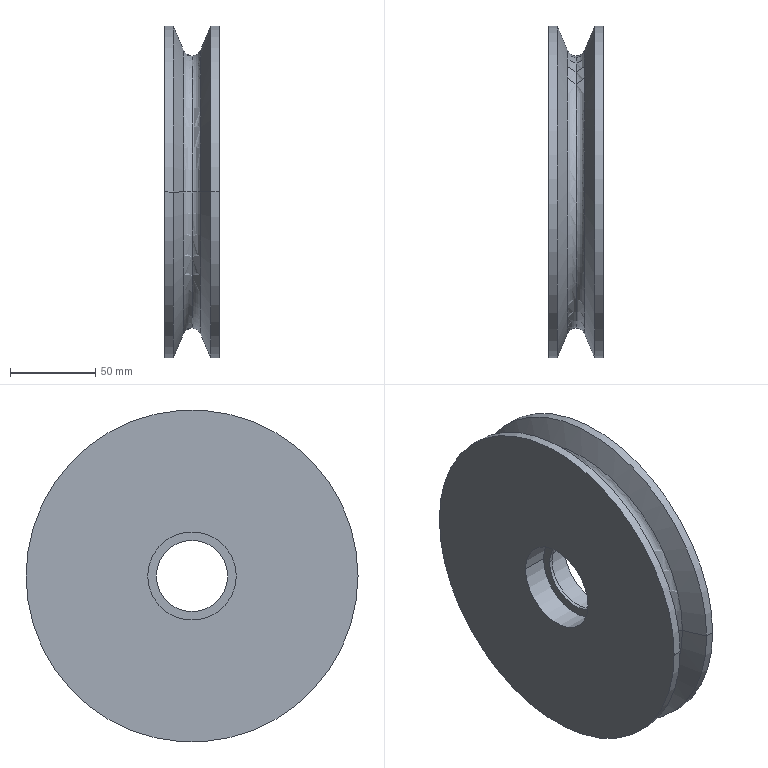Part | SolidWorks | features ICE 2, MirrorPattern 1, Revolution 1 | 1 solid | 22 faces | box 32 x 195 x 195 mm | volume 746203 mm3 | cylinder 10 | torus 4 | cone 4 | plane 4 | commonest cylinder face diameters 52 x4 195 x4 42 x2
STEP:
#1=CARTESIAN_POINT('',(5.072,83.372,0.));
#2=VERTEX_POINT('',#1);
#3=CARTESIAN_POINT('',(0.,80.,0.));
#4=VERTEX_POINT('',#3);
#5=CARTESIAN_POINT('',(0.,85.5,0.));
#6=DIRECTION('',(0.,0.,-1.));
#7=DIRECTION('',(-1.,0.,0.));
#8=AXIS2_PLACEMENT_3D('',#5,#6,#7);
#9=CIRCLE('',#8,5.5);
#10=EDGE_CURVE('',#2,#4,#9,.T.);
#11=ORIENTED_EDGE('',*,*,#10,.T.);
#12=CARTESIAN_POINT('',(0.,-80.,0.));
#13=VERTEX_POINT('',#12);
#14=CARTESIAN_POINT('',(0.,0.,0.));
#15=DIRECTION('',(1.,0.,0.));
#16=DIRECTION('',(0.,1.,0.));
#17=AXIS2_PLACEMENT_3D('',#14,#15,#16);
#18=CIRCLE('',#17,80.);
#19=EDGE_CURVE('',#4,#13,#18,.T.);
#20=ORIENTED_EDGE('',*,*,#19,.T.);
#21=CARTESIAN_POINT('',(5.072,-83.372,0.));
#22=VERTEX_POINT('',#21);
#23=CARTESIAN_POINT('',(0.,-85.5,0.));
#24=DIRECTION('',(0.,0.,1.));
#25=DIRECTION('',(0.,-1.,0.));
#26=AXIS2_PLACEMENT_3D('',#23,#24,#25);
#27=CIRCLE('',#26,5.5);
#28=EDGE_CURVE('',#22,#13,#27,.T.);
#29=ORIENTED_EDGE('',*,*,#28,.F.);
#30=CARTESIAN_POINT('',(5.072,0.,0.));
#31=DIRECTION('',(1.,0.,0.));
#32=DIRECTION('',(0.,1.,0.));
#33=AXIS2_PLACEMENT_3D('',#30,#31,#32);
#34=CIRCLE('',#33,83.372);
#35=EDGE_CURVE('',#2,#22,#34,.T.);
#36=ORIENTED_EDGE('',*,*,#35,.F.);
#37=EDGE_LOOP('',(#11,#20,#29,#36));
#38=FACE_OUTER_BOUND('',#37,.T.);
#39=CARTESIAN_POINT('',(0.,0.,0.));
#40=DIRECTION('',(1.,0.,0.));
#41=DIRECTION('',(0.,1.,0.));
#42=AXIS2_PLACEMENT_3D('',#39,#40,#41);
#43=TOROIDAL_SURFACE('',#42,85.5,5.5);
#44=ADVANCED_FACE('',(#38),#43,.F.);
#45=ORIENTED_EDGE('',*,*,#28,.T.);
#46=CARTESIAN_POINT('',(0.,0.,0.));
#47=DIRECTION('',(1.,0.,0.));
#48=DIRECTION('',(0.,1.,0.));
#49=AXIS2_PLACEMENT_3D('',#46,#47,#48);
#50=CIRCLE('',#49,80.);
#51=EDGE_CURVE('',#13,#4,#50,.T.);
#52=ORIENTED_EDGE('',*,*,#51,.T.);
#53=ORIENTED_EDGE('',*,*,#10,.F.);
#54=CARTESIAN_POINT('',(5.072,0.,0.));
#55=DIRECTION('',(1.,0.,0.));
#56=DIRECTION('',(0.,1.,0.));
#57=AXIS2_PLACEMENT_3D('',#54,#55,#56);
#58=CIRCLE('',#57,83.372);
#59=EDGE_CURVE('',#22,#2,#58,.T.);
#60=ORIENTED_EDGE('',*,*,#59,.F.);
#61=EDGE_LOOP('',(#45,#52,#53,#60));
#62=FACE_OUTER_BOUND('',#61,.T.);
#63=CARTESIAN_POINT('',(0.,0.,0.));
#64=DIRECTION('',(1.,0.,0.));
#65=DIRECTION('',(0.,1.,0.));
#66=AXIS2_PLACEMENT_3D('',#63,#64,#65);
#67=TOROIDAL_SURFACE('',#66,85.5,5.5);
#68=ADVANCED_FACE('',(#62),#67,.F.);
#69=CARTESIAN_POINT('',(-1.,-26.,0.));
#70=VERTEX_POINT('',#69);
#71=CARTESIAN_POINT('',(-1.,26.,0.));
#72=VERTEX_POINT('',#71);
#73=CARTESIAN_POINT('',(-1.,0.,0.));
#74=DIRECTION('',(1.,0.,0.));
#75=DIRECTION('',(0.,1.,0.));
#76=AXIS2_PLACEMENT_3D('',#73,#74,#75);
#77=CIRCLE('',#76,26.);
#78=EDGE_CURVE('',#70,#72,#77,.T.);
#79=ORIENTED_EDGE('',*,*,#78,.T.);
#80=CARTESIAN_POINT('',(-16.,26.,0.));
#81=VERTEX_POINT('',#80);
#82=CARTESIAN_POINT('',(-1.,26.,0.));
#83=DIRECTION('',(-1.,0.,0.));
#84=VECTOR('',#83,1000.);
#85=LINE('',#82,#84);
#86=EDGE_CURVE('',#72,#81,#85,.T.);
#87=ORIENTED_EDGE('',*,*,#86,.T.);
#88=CARTESIAN_POINT('',(-16.,-26.,0.));
#89=VERTEX_POINT('',#88);
#90=CARTESIAN_POINT('',(-16.,0.,0.));
#91=DIRECTION('',(1.,0.,0.));
#92=DIRECTION('',(0.,1.,0.));
#93=AXIS2_PLACEMENT_3D('',#90,#91,#92);
#94=CIRCLE('',#93,26.);
#95=EDGE_CURVE('',#89,#81,#94,.T.);
#96=ORIENTED_EDGE('',*,*,#95,.F.);
#97=CARTESIAN_POINT('',(-1.,-26.,0.));
#98=DIRECTION('',(-1.,0.,0.));
#99=VECTOR('',#98,1000.);
#100=LINE('',#97,#99);
#101=EDGE_CURVE('',#70,#89,#100,.T.);
#102=ORIENTED_EDGE('',*,*,#101,.F.);
#103=EDGE_LOOP('',(#79,#87,#96,#102));
#104=FACE_OUTER_BOUND('',#103,.T.);
#105=CARTESIAN_POINT('',(-1.,0.,0.));
#106=DIRECTION('',(-1.,0.,0.));
#107=DIRECTION('',(0.,-1.,0.));
#108=AXIS2_PLACEMENT_3D('',#105,#106,#107);
#109=CYLINDRICAL_SURFACE('',#108,26.);
#110=ADVANCED_FACE('',(#104),#109,.F.);
#111=CARTESIAN_POINT('',(1.,-26.,0.));
#112=VERTEX_POINT('',#111);
#113=CARTESIAN_POINT('',(1.,26.,0.));
#114=VERTEX_POINT('',#113);
#115=CARTESIAN_POINT('',(1.,0.,0.));
#116=DIRECTION('',(1.,0.,0.));
#117=DIRECTION('',(0.,1.,0.));
#118=AXIS2_PLACEMENT_3D('',#115,#116,#117);
#119=CIRCLE('',#118,26.);
#120=EDGE_CURVE('',#112,#114,#119,.T.);
#121=ORIENTED_EDGE('',*,*,#120,.F.);
#122=CARTESIAN_POINT('',(16.,-26.,0.));
#123=VERTEX_POINT('',#122);
#124=CARTESIAN_POINT('',(1.,-26.,0.));
#125=DIRECTION('',(1.,0.,0.));
#126=VECTOR('',#125,1000.);
#127=LINE('',#124,#126);
#128=EDGE_CURVE('',#112,#123,#127,.T.);
#129=ORIENTED_EDGE('',*,*,#128,.T.);
#130=CARTESIAN_POINT('',(16.,26.,0.));
#131=VERTEX_POINT('',#130);
#132=CARTESIAN_POINT('',(16.,0.,0.));
#133=DIRECTION('',(1.,0.,0.));
#134=DIRECTION('',(0.,1.,0.));
#135=AXIS2_PLACEMENT_3D('',#132,#133,#134);
#136=CIRCLE('',#135,26.);
#137=EDGE_CURVE('',#123,#131,#136,.T.);
#138=ORIENTED_EDGE('',*,*,#137,.T.);
#139=CARTESIAN_POINT('',(1.,26.,0.));
#140=DIRECTION('',(1.,0.,0.));
#141=VECTOR('',#140,1000.);
#142=LINE('',#139,#141);
#143=EDGE_CURVE('',#114,#131,#142,.T.);
#144=ORIENTED_EDGE('',*,*,#143,.F.);
#145=EDGE_LOOP('',(#121,#129,#138,#144));
#146=FACE_OUTER_BOUND('',#145,.T.);
#147=CARTESIAN_POINT('',(1.,0.,0.));
#148=DIRECTION('',(1.,0.,0.));
#149=DIRECTION('',(0.,1.,0.));
#150=AXIS2_PLACEMENT_3D('',#147,#148,#149);
#151=CYLINDRICAL_SURFACE('',#150,26.);
#152=ADVANCED_FACE('',(#146),#151,.F.);
#153=CARTESIAN_POINT('',(-16.,97.5,0.));
#154=VERTEX_POINT('',#153);
#155=CARTESIAN_POINT('',(-16.,-97.5,0.));
#156=VERTEX_POINT('',#155);
#157=CARTESIAN_POINT('',(-16.,0.,0.));
#158=DIRECTION('',(1.,0.,0.));
#159=DIRECTION('',(0.,1.,0.));
#160=AXIS2_PLACEMENT_3D('',#157,#158,#159);
#161=CIRCLE('',#160,97.5);
#162=EDGE_CURVE('',#154,#156,#161,.T.);
#163=ORIENTED_EDGE('',*,*,#162,.T.);
#164=CARTESIAN_POINT('',(-11.,-97.5,0.));
#165=VERTEX_POINT('',#164);
#166=CARTESIAN_POINT('',(16.,-97.5,0.));
#167=DIRECTION('',(1.,0.,0.));
#168=VECTOR('',#167,1000.);
#169=LINE('',#166,#168);
#170=EDGE_CURVE('',#156,#165,#169,.T.);
#171=ORIENTED_EDGE('',*,*,#170,.T.);
#172=CARTESIAN_POINT('',(-11.,97.5,0.));
#173=VERTEX_POINT('',#172);
#174=CARTESIAN_POINT('',(-11.,0.,0.));
#175=DIRECTION('',(1.,0.,0.));
#176=DIRECTION('',(0.,1.,0.));
#177=AXIS2_PLACEMENT_3D('',#174,#175,#176);
#178=CIRCLE('',#177,97.5);
#179=EDGE_CURVE('',#173,#165,#178,.T.);
#180=ORIENTED_EDGE('',*,*,#179,.F.);
#181=CARTESIAN_POINT('',(16.,97.5,0.));
#182=DIRECTION('',(1.,0.,0.));
#183=VECTOR('',#182,1000.);
#184=LINE('',#181,#183);
#185=EDGE_CURVE('',#154,#173,#184,.T.);
#186=ORIENTED_EDGE('',*,*,#185,.F.);
#187=EDGE_LOOP('',(#163,#171,#180,#186));
#188=FACE_OUTER_BOUND('',#187,.T.);
#189=CARTESIAN_POINT('',(16.,0.,0.));
#190=DIRECTION('',(1.,0.,0.));
#191=DIRECTION('',(0.,1.,0.));
#192=AXIS2_PLACEMENT_3D('',#189,#190,#191);
#193=CYLINDRICAL_SURFACE('',#192,97.5);
#194=ADVANCED_FACE('',(#188),#193,.T.);
#195=CARTESIAN_POINT('',(-5.072,83.372,0.));
#196=VERTEX_POINT('',#195);
#197=CARTESIAN_POINT('',(-5.072,-83.372,0.));
#198=VERTEX_POINT('',#197);
#199=CARTESIAN_POINT('',(-5.072,0.,0.));
#200=DIRECTION('',(1.,0.,0.));
#201=DIRECTION('',(0.,1.,0.));
#202=AXIS2_PLACEMENT_3D('',#199,#200,#201);
#203=CIRCLE('',#202,83.372);
#204=EDGE_CURVE('',#196,#198,#203,.T.);
#205=ORIENTED_EDGE('',*,*,#204,.F.);
#206=CARTESIAN_POINT('',(-5.072,83.372,0.));
#207=DIRECTION('',(-0.3869,0.9221,0.));
#208=VECTOR('',#207,1000.);
#209=LINE('',#206,#208);
#210=EDGE_CURVE('',#196,#173,#209,.T.);
#211=ORIENTED_EDGE('',*,*,#210,.T.);
#212=ORIENTED_EDGE('',*,*,#179,.T.);
#213=CARTESIAN_POINT('',(-5.072,-83.372,0.));
#214=DIRECTION('',(-0.3869,-0.9221,0.));
#215=VECTOR('',#214,1000.);
#216=LINE('',#213,#215);
#217=EDGE_CURVE('',#198,#165,#216,.T.);
#218=ORIENTED_EDGE('',*,*,#217,.F.);
#219=EDGE_LOOP('',(#205,#211,#212,#218));
#220=FACE_OUTER_BOUND('',#219,.T.);
#221=CARTESIAN_POINT('',(-5.072,0.,0.));
#222=DIRECTION('',(-1.,0.,0.));
#223=DIRECTION('',(0.,-1.,0.));
#224=AXIS2_PLACEMENT_3D('',#221,#222,#223);
#225=CONICAL_SURFACE('',#224,83.372,1.173);
#226=ADVANCED_FACE('',(#220),#225,.T.);
#227=ORIENTED_EDGE('',*,*,#51,.F.);
#228=CARTESIAN_POINT('',(0.,-85.5,0.));
#229=DIRECTION('',(0.,0.,1.));
#230=DIRECTION('',(0.,-1.,0.));
#231=AXIS2_PLACEMENT_3D('',#228,#229,#230);
#232=CIRCLE('',#231,5.5);
#233=EDGE_CURVE('',#13,#198,#232,.T.);
#234=ORIENTED_EDGE('',*,*,#233,.T.);
#235=CARTESIAN_POINT('',(-5.072,0.,0.));
#236=DIRECTION('',(1.,0.,0.));
#237=DIRECTION('',(0.,1.,0.));
#238=AXIS2_PLACEMENT_3D('',#235,#236,#237);
#239=CIRCLE('',#238,83.372);
#240=EDGE_CURVE('',#198,#196,#239,.T.);
#241=ORIENTED_EDGE('',*,*,#240,.T.);
#242=CARTESIAN_POINT('',(0.,85.5,0.));
#243=DIRECTION('',(0.,0.,-1.));
#244=DIRECTION('',(-1.,0.,0.));
#245=AXIS2_PLACEMENT_3D('',#242,#243,#244);
#246=CIRCLE('',#245,5.5);
#247=EDGE_CURVE('',#4,#196,#246,.T.);
#248=ORIENTED_EDGE('',*,*,#247,.F.);
#249=EDGE_LOOP('',(#227,#234,#241,#248));
#250=FACE_OUTER_BOUND('',#249,.T.);
#251=CARTESIAN_POINT('',(0.,0.,0.));
#252=DIRECTION('',(1.,0.,0.));
#253=DIRECTION('',(0.,1.,0.));
#254=AXIS2_PLACEMENT_3D('',#251,#252,#253);
#255=TOROIDAL_SURFACE('',#254,85.5,5.5);
#256=ADVANCED_FACE('',(#250),#255,.F.);
#257=ORIENTED_EDGE('',*,*,#35,.T.);
#258=CARTESIAN_POINT('',(11.,-97.5,0.));
#259=VERTEX_POINT('',#258);
#260=CARTESIAN_POINT('',(11.,-97.5,0.));
#261=DIRECTION('',(0.3869,-0.9221,0.));
#262=VECTOR('',#261,1000.);
#263=LINE('',#260,#262);
#264=EDGE_CURVE('',#22,#259,#263,.T.);
#265=ORIENTED_EDGE('',*,*,#264,.T.);
#266=CARTESIAN_POINT('',(11.,97.5,0.));
#267=VERTEX_POINT('',#266);
#268=CARTESIAN_POINT('',(11.,0.,0.));
#269=DIRECTION('',(1.,0.,0.));
#270=DIRECTION('',(0.,1.,0.));
#271=AXIS2_PLACEMENT_3D('',#268,#269,#270);
#272=CIRCLE('',#271,97.5);
#273=EDGE_CURVE('',#267,#259,#272,.T.);
#274=ORIENTED_EDGE('',*,*,#273,.F.);
#275=CARTESIAN_POINT('',(11.,97.5,0.));
#276=DIRECTION('',(0.3869,0.9221,0.));
#277=VECTOR('',#276,1000.);
#278=LINE('',#275,#277);
#279=EDGE_CURVE('',#2,#267,#278,.T.);
#280=ORIENTED_EDGE('',*,*,#279,.F.);
#281=EDGE_LOOP('',(#257,#265,#274,#280));
#282=FACE_OUTER_BOUND('',#281,.T.);
#283=CARTESIAN_POINT('',(11.,0.,0.));
#284=DIRECTION('',(1.,0.,0.));
#285=DIRECTION('',(0.,1.,0.));
#286=AXIS2_PLACEMENT_3D('',#283,#284,#285);
#287=CONICAL_SURFACE('',#286,97.5,1.173);
#288=ADVANCED_FACE('',(#282),#287,.T.);
#289=ORIENTED_EDGE('',*,*,#273,.T.);
#290=CARTESIAN_POINT('',(16.,-97.5,0.));
#291=VERTEX_POINT('',#290);
#292=CARTESIAN_POINT('',(16.,-97.5,0.));
#293=DIRECTION('',(1.,0.,0.));
#294=VECTOR('',#293,1000.);
#295=LINE('',#292,#294);
#296=EDGE_CURVE('',#259,#291,#295,.T.);
#297=ORIENTED_EDGE('',*,*,#296,.T.);
#298=CARTESIAN_POINT('',(16.,97.5,0.));
#299=VERTEX_POINT('',#298);
#300=CARTESIAN_POINT('',(16.,0.,0.));
#301=DIRECTION('',(1.,0.,0.));
#302=DIRECTION('',(0.,1.,0.));
#303=AXIS2_PLACEMENT_3D('',#300,#301,#302);
#304=CIRCLE('',#303,97.5);
#305=EDGE_CURVE('',#299,#291,#304,.T.);
#306=ORIENTED_EDGE('',*,*,#305,.F.);
#307=CARTESIAN_POINT('',(16.,97.5,0.));
#308=DIRECTION('',(1.,0.,0.));
#309=VECTOR('',#308,1000.);
#310=LINE('',#307,#309);
#311=EDGE_CURVE('',#267,#299,#310,.T.);
#312=ORIENTED_EDGE('',*,*,#311,.F.);
#313=EDGE_LOOP('',(#289,#297,#306,#312));
#314=FACE_OUTER_BOUND('',#313,.T.);
#315=CARTESIAN_POINT('',(16.,0.,0.));
#316=DIRECTION('',(1.,0.,0.));
#317=DIRECTION('',(0.,1.,0.));
#318=AXIS2_PLACEMENT_3D('',#315,#316,#317);
#319=CYLINDRICAL_SURFACE('',#318,97.5);
#320=ADVANCED_FACE('',(#314),#319,.T.);
#321=CARTESIAN_POINT('',(-1.,-21.,0.));
#322=VERTEX_POINT('',#321);
#323=CARTESIAN_POINT('',(-1.,21.,0.));
#324=VERTEX_POINT('',#323);
#325=CARTESIAN_POINT('',(-1.,0.,0.));
#326=DIRECTION('',(1.,0.,0.));
#327=DIRECTION('',(0.,-1.,0.));
#328=AXIS2_PLACEMENT_3D('',#325,#326,#327);
#329=CIRCLE('',#328,21.);
#330=EDGE_CURVE('',#322,#324,#329,.T.);
#331=ORIENTED_EDGE('',*,*,#330,.F.);
#332=CARTESIAN_POINT('',(1.,-21.,0.));
#333=VERTEX_POINT('',#332);
#334=CARTESIAN_POINT('',(-16.001,-21.,0.));
#335=DIRECTION('',(1.,0.,0.));
#336=VECTOR('',#335,1000.);
#337=LINE('',#334,#336);
#338=EDGE_CURVE('',#322,#333,#337,.T.);
#339=ORIENTED_EDGE('',*,*,#338,.T.);
#340=CARTESIAN_POINT('',(1.,21.,0.));
#341=VERTEX_POINT('',#340);
#342=CARTESIAN_POINT('',(1.,0.,0.));
#343=DIRECTION('',(-1.,0.,0.));
#344=DIRECTION('',(0.,1.,0.));
#345=AXIS2_PLACEMENT_3D('',#342,#343,#344);
#346=CIRCLE('',#345,21.);
#347=EDGE_CURVE('',#341,#333,#346,.T.);
#348=ORIENTED_EDGE('',*,*,#347,.F.);
#349=CARTESIAN_POINT('',(-16.001,21.,0.));
#350=DIRECTION('',(1.,0.,0.));
#351=VECTOR('',#350,1000.);
#352=LINE('',#349,#351);
#353=EDGE_CURVE('',#324,#341,#352,.T.);
#354=ORIENTED_EDGE('',*,*,#353,.F.);
#355=EDGE_LOOP('',(#331,#339,#348,#354));
#356=FACE_OUTER_BOUND('',#355,.T.);
#357=CARTESIAN_POINT('',(-16.001,0.,0.));
#358=DIRECTION('',(1.,0.,0.));
#359=DIRECTION('',(0.,1.,0.));
#360=AXIS2_PLACEMENT_3D('',#357,#358,#359);
#361=CYLINDRICAL_SURFACE('',#360,21.);
#362=ADVANCED_FACE('',(#356),#361,.F.);
#363=ORIENTED_EDGE('',*,*,#338,.F.);
#364=CARTESIAN_POINT('',(-1.,0.,0.));
#365=DIRECTION('',(1.,0.,0.));
#366=DIRECTION('',(0.,-1.,0.));
#367=AXIS2_PLACEMENT_3D('',#364,#365,#366);
#368=CIRCLE('',#367,21.);
#369=EDGE_CURVE('',#324,#322,#368,.T.);
#370=ORIENTED_EDGE('',*,*,#369,.F.);
#371=ORIENTED_EDGE('',*,*,#353,.T.);
#372=CARTESIAN_POINT('',(1.,0.,0.));
#373=DIRECTION('',(-1.,0.,0.));
#374=DIRECTION('',(0.,1.,0.));
#375=AXIS2_PLACEMENT_3D('',#372,#373,#374);
#376=CIRCLE('',#375,21.);
#377=EDGE_CURVE('',#333,#341,#376,.T.);
#378=ORIENTED_EDGE('',*,*,#377,.F.);
#379=EDGE_LOOP('',(#363,#370,#371,#378));
#380=FACE_OUTER_BOUND('',#379,.T.);
#381=CARTESIAN_POINT('',(-16.001,0.,0.));
#382=DIRECTION('',(1.,0.,0.));
#383=DIRECTION('',(0.,1.,0.));
#384=AXIS2_PLACEMENT_3D('',#381,#382,#383);
#385=CYLINDRICAL_SURFACE('',#384,21.);
#386=ADVANCED_FACE('',(#380),#385,.F.);
#387=CARTESIAN_POINT('',(16.,0.,0.));
#388=DIRECTION('',(1.,0.,0.));
#389=DIRECTION('',(0.,1.,0.));
#390=AXIS2_PLACEMENT_3D('',#387,#388,#389);
#391=CIRCLE('',#390,26.);
#392=EDGE_CURVE('',#131,#123,#391,.T.);
#393=ORIENTED_EDGE('',*,*,#392,.F.);
#394=ORIENTED_EDGE('',*,*,#137,.F.);
#395=EDGE_LOOP('',(#393,#394));
#396=FACE_BOUND('',#395,.T.);
#397=ORIENTED_EDGE('',*,*,#305,.T.);
#398=CARTESIAN_POINT('',(16.,0.,0.));
#399=DIRECTION('',(1.,0.,0.));
#400=DIRECTION('',(0.,1.,0.));
#401=AXIS2_PLACEMENT_3D('',#398,#399,#400);
#402=CIRCLE('',#401,97.5);
#403=EDGE_CURVE('',#291,#299,#402,.T.);
#404=ORIENTED_EDGE('',*,*,#403,.T.);
#405=EDGE_LOOP('',(#397,#404));
#406=FACE_OUTER_BOUND('',#405,.T.);
#407=CARTESIAN_POINT('',(16.,0.,0.));
#408=DIRECTION('',(1.,0.,0.));
#409=DIRECTION('',(0.,1.,0.));
#410=AXIS2_PLACEMENT_3D('',#407,#408,#409);
#411=PLANE('',#410);
#412=ADVANCED_FACE('',(#396,#406),#411,.T.);
#413=ORIENTED_EDGE('',*,*,#296,.F.);
#414=CARTESIAN_POINT('',(11.,0.,0.));
#415=DIRECTION('',(1.,0.,0.));
#416=DIRECTION('',(0.,1.,0.));
#417=AXIS2_PLACEMENT_3D('',#414,#415,#416);
#418=CIRCLE('',#417,97.5);
#419=EDGE_CURVE('',#259,#267,#418,.T.);
#420=ORIENTED_EDGE('',*,*,#419,.T.);
#421=ORIENTED_EDGE('',*,*,#311,.T.);
#422=ORIENTED_EDGE('',*,*,#403,.F.);
#423=EDGE_LOOP('',(#413,#420,#421,#422));
#424=FACE_OUTER_BOUND('',#423,.T.);
#425=CARTESIAN_POINT('',(16.,0.,0.));
#426=DIRECTION('',(1.,0.,0.));
#427=DIRECTION('',(0.,1.,0.));
#428=AXIS2_PLACEMENT_3D('',#425,#426,#427);
#429=CYLINDRICAL_SURFACE('',#428,97.5);
#430=ADVANCED_FACE('',(#424),#429,.T.);
#431=ORIENTED_EDGE('',*,*,#264,.F.);
#432=ORIENTED_EDGE('',*,*,#59,.T.);
#433=ORIENTED_EDGE('',*,*,#279,.T.);
#434=ORIENTED_EDGE('',*,*,#419,.F.);
#435=EDGE_LOOP('',(#431,#432,#433,#434));
#436=FACE_OUTER_BOUND('',#435,.T.);
#437=CARTESIAN_POINT('',(11.,0.,0.));
#438=DIRECTION('',(1.,0.,0.));
#439=DIRECTION('',(0.,1.,0.));
#440=AXIS2_PLACEMENT_3D('',#437,#438,#439);
#441=CONICAL_SURFACE('',#440,97.5,1.173);
#442=ADVANCED_FACE('',(#436),#441,.T.);
#443=ORIENTED_EDGE('',*,*,#19,.F.);
#444=ORIENTED_EDGE('',*,*,#247,.T.);
#445=ORIENTED_EDGE('',*,*,#204,.T.);
#446=ORIENTED_EDGE('',*,*,#233,.F.);
#447=EDGE_LOOP('',(#443,#444,#445,#446));
#448=FACE_OUTER_BOUND('',#447,.T.);
#449=CARTESIAN_POINT('',(0.,0.,0.));
#450=DIRECTION('',(1.,0.,0.));
#451=DIRECTION('',(0.,1.,0.));
#452=AXIS2_PLACEMENT_3D('',#449,#450,#451);
#453=TOROIDAL_SURFACE('',#452,85.5,5.5);
#454=ADVANCED_FACE('',(#448),#453,.F.);
#455=ORIENTED_EDGE('',*,*,#210,.F.);
#456=ORIENTED_EDGE('',*,*,#240,.F.);
#457=ORIENTED_EDGE('',*,*,#217,.T.);
#458=CARTESIAN_POINT('',(-11.,0.,0.));
#459=DIRECTION('',(1.,0.,0.));
#460=DIRECTION('',(0.,1.,0.));
#461=AXIS2_PLACEMENT_3D('',#458,#459,#460);
#462=CIRCLE('',#461,97.5);
#463=EDGE_CURVE('',#165,#173,#462,.T.);
#464=ORIENTED_EDGE('',*,*,#463,.T.);
#465=EDGE_LOOP('',(#455,#456,#457,#464));
#466=FACE_OUTER_BOUND('',#465,.T.);
#467=CARTESIAN_POINT('',(-5.072,0.,0.));
#468=DIRECTION('',(-1.,0.,0.));
#469=DIRECTION('',(0.,-1.,0.));
#470=AXIS2_PLACEMENT_3D('',#467,#468,#469);
#471=CONICAL_SURFACE('',#470,83.372,1.173);
#472=ADVANCED_FACE('',(#466),#471,.T.);
#473=ORIENTED_EDGE('',*,*,#170,.F.);
#474=CARTESIAN_POINT('',(-16.,0.,0.));
#475=DIRECTION('',(1.,0.,0.));
#476=DIRECTION('',(0.,1.,0.));
#477=AXIS2_PLACEMENT_3D('',#474,#475,#476);
#478=CIRCLE('',#477,97.5);
#479=EDGE_CURVE('',#156,#154,#478,.T.);
#480=ORIENTED_EDGE('',*,*,#479,.T.);
#481=ORIENTED_EDGE('',*,*,#185,.T.);
#482=ORIENTED_EDGE('',*,*,#463,.F.);
#483=EDGE_LOOP('',(#473,#480,#481,#482));
#484=FACE_OUTER_BOUND('',#483,.T.);
#485=CARTESIAN_POINT('',(16.,0.,0.));
#486=DIRECTION('',(1.,0.,0.));
#487=DIRECTION('',(0.,1.,0.));
#488=AXIS2_PLACEMENT_3D('',#485,#486,#487);
#489=CYLINDRICAL_SURFACE('',#488,97.5);
#490=ADVANCED_FACE('',(#484),#489,.T.);
#491=ORIENTED_EDGE('',*,*,#95,.T.);
#492=CARTESIAN_POINT('',(-16.,0.,0.));
#493=DIRECTION('',(1.,0.,0.));
#494=DIRECTION('',(0.,1.,0.));
#495=AXIS2_PLACEMENT_3D('',#492,#493,#494);
#496=CIRCLE('',#495,26.);
#497=EDGE_CURVE('',#81,#89,#496,.T.);
#498=ORIENTED_EDGE('',*,*,#497,.T.);
#499=EDGE_LOOP('',(#491,#498));
#500=FACE_BOUND('',#499,.T.);
#501=ORIENTED_EDGE('',*,*,#162,.F.);
#502=ORIENTED_EDGE('',*,*,#479,.F.);
#503=EDGE_LOOP('',(#501,#502));
#504=FACE_OUTER_BOUND('',#503,.T.);
#505=CARTESIAN_POINT('',(-16.,0.,0.));
#506=DIRECTION('',(-1.,0.,0.));
#507=DIRECTION('',(0.,-1.,0.));
#508=AXIS2_PLACEMENT_3D('',#505,#506,#507);
#509=PLANE('',#508);
#510=ADVANCED_FACE('',(#500,#504),#509,.T.);
#511=CARTESIAN_POINT('',(1.,0.,0.));
#512=DIRECTION('',(1.,0.,0.));
#513=DIRECTION('',(0.,1.,0.));
#514=AXIS2_PLACEMENT_3D('',#511,#512,#513);
#515=CIRCLE('',#514,26.);
#516=EDGE_CURVE('',#114,#112,#515,.T.);
#517=ORIENTED_EDGE('',*,*,#516,.T.);
#518=ORIENTED_EDGE('',*,*,#120,.T.);
#519=EDGE_LOOP('',(#517,#518));
#520=FACE_OUTER_BOUND('',#519,.T.);
#521=ORIENTED_EDGE('',*,*,#347,.T.);
#522=ORIENTED_EDGE('',*,*,#377,.T.);
#523=EDGE_LOOP('',(#521,#522));
#524=FACE_BOUND('',#523,.T.);
#525=CARTESIAN_POINT('',(1.,0.,0.));
#526=DIRECTION('',(1.,0.,0.));
#527=DIRECTION('',(0.,1.,0.));
#528=AXIS2_PLACEMENT_3D('',#525,#526,#527);
#529=PLANE('',#528);
#530=ADVANCED_FACE('',(#520,#524),#529,.T.);
#531=ORIENTED_EDGE('',*,*,#128,.F.);
#532=ORIENTED_EDGE('',*,*,#516,.F.);
#533=ORIENTED_EDGE('',*,*,#143,.T.);
#534=ORIENTED_EDGE('',*,*,#392,.T.);
#535=EDGE_LOOP('',(#531,#532,#533,#534));
#536=FACE_OUTER_BOUND('',#535,.T.);
#537=CARTESIAN_POINT('',(1.,0.,0.));
#538=DIRECTION('',(1.,0.,0.));
#539=DIRECTION('',(0.,1.,0.));
#540=AXIS2_PLACEMENT_3D('',#537,#538,#539);
#541=CYLINDRICAL_SURFACE('',#540,26.);
#542=ADVANCED_FACE('',(#536),#541,.F.);
#543=ORIENTED_EDGE('',*,*,#78,.F.);
#544=CARTESIAN_POINT('',(-1.,0.,0.));
#545=DIRECTION('',(1.,0.,0.));
#546=DIRECTION('',(0.,1.,0.));
#547=AXIS2_PLACEMENT_3D('',#544,#545,#546);
#548=CIRCLE('',#547,26.);
#549=EDGE_CURVE('',#72,#70,#548,.T.);
#550=ORIENTED_EDGE('',*,*,#549,.F.);
#551=EDGE_LOOP('',(#543,#550));
#552=FACE_OUTER_BOUND('',#551,.T.);
#553=ORIENTED_EDGE('',*,*,#369,.T.);
#554=ORIENTED_EDGE('',*,*,#330,.T.);
#555=EDGE_LOOP('',(#553,#554));
#556=FACE_BOUND('',#555,.T.);
#557=CARTESIAN_POINT('',(-1.,0.,0.));
#558=DIRECTION('',(-1.,0.,0.));
#559=DIRECTION('',(0.,1.,0.));
#560=AXIS2_PLACEMENT_3D('',#557,#558,#559);
#561=PLANE('',#560);
#562=ADVANCED_FACE('',(#552,#556),#561,.T.);
#563=ORIENTED_EDGE('',*,*,#86,.F.);
#564=ORIENTED_EDGE('',*,*,#549,.T.);
#565=ORIENTED_EDGE('',*,*,#101,.T.);
#566=ORIENTED_EDGE('',*,*,#497,.F.);
#567=EDGE_LOOP('',(#563,#564,#565,#566));
#568=FACE_OUTER_BOUND('',#567,.T.);
#569=CARTESIAN_POINT('',(-1.,0.,0.));
#570=DIRECTION('',(-1.,0.,0.));
#571=DIRECTION('',(0.,-1.,0.));
#572=AXIS2_PLACEMENT_3D('',#569,#570,#571);
#573=CYLINDRICAL_SURFACE('',#572,26.);
#574=ADVANCED_FACE('',(#568),#573,.F.);
#575=CLOSED_SHELL('',(#44,#68,#110,#152,#194,#226,#256,#288,#320,#362,#386,#412,#430,#442,#454,#472,#490,#510,#530,#542,#562,#574));
#576=MANIFOLD_SOLID_BREP('',#575);
#577=CARTESIAN_POINT('',(0.,0.,0.));
#578=DIRECTION('',(0.,0.,1.));
#579=DIRECTION('',(1.,0.,0.));
#580=AXIS2_PLACEMENT_3D('',#577,#578,#579);
#581=(LENGTH_UNIT()NAMED_UNIT(*)SI_UNIT(.MILLI.,.METRE.));
#582=UNCERTAINTY_MEASURE_WITH_UNIT(LENGTH_MEASURE(0.00001),#581,'','');
#583=(NAMED_UNIT(*)PLANE_ANGLE_UNIT()SI_UNIT($,.RADIAN.));
#584=(NAMED_UNIT(*)SI_UNIT($,.STERADIAN.)SOLID_ANGLE_UNIT());
#585=(GEOMETRIC_REPRESENTATION_CONTEXT(3)GLOBAL_UNCERTAINTY_ASSIGNED_CONTEXT((#582))GLOBAL_UNIT_ASSIGNED_CONTEXT((#581,#583,#584))REPRESENTATION_CONTEXT('',''));
#586=ADVANCED_BREP_SHAPE_REPRESENTATION('',(#576,#580),#585);